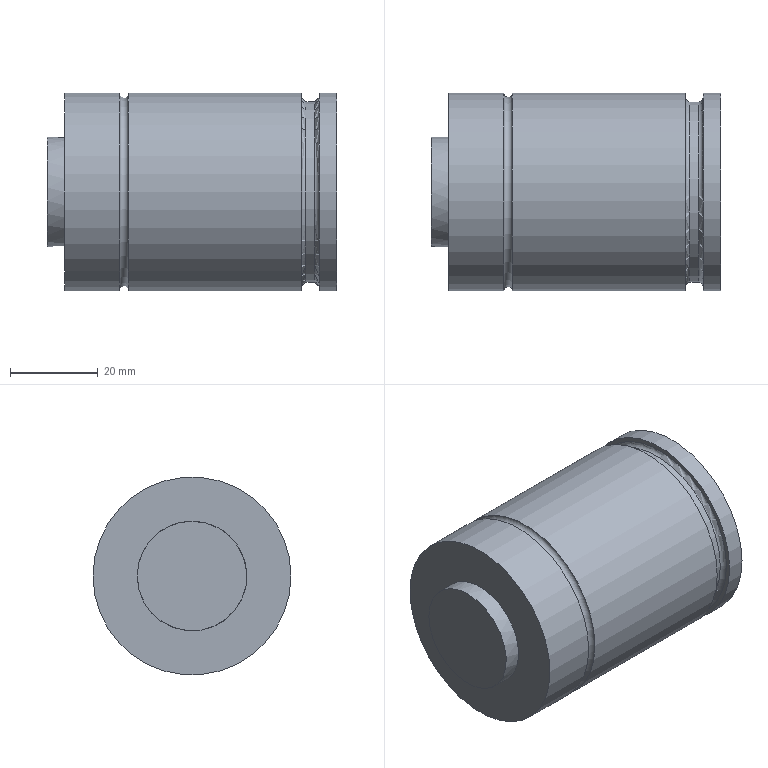Part | NX | features solid 2 | 1 solid | 17 faces | box 66 x 45.2 x 45.2 mm | volume 98109 mm3 | cylinder 7 | plane 5 | torus 3 | cone 2 | commonest cylinder face diameters 45.2 x3 8 x2 25 x1 41.2 x1
STEP:
#1=CARTESIAN_POINT('',(-246.5,-282.6,170.));
#2=VERTEX_POINT('',#1);
#3=CARTESIAN_POINT('',(-246.5,-260.,170.));
#4=DIRECTION('',(1.,0.,0.));
#5=DIRECTION('',(0.,-1.,0.));
#6=AXIS2_PLACEMENT_3D('',#3,#4,#5);
#7=CIRCLE('',#6,22.6);
#8=EDGE_CURVE('',#2,#2,#7,.T.);
#9=ORIENTED_EDGE('',*,*,#8,.T.);
#10=EDGE_LOOP('',(#9));
#11=FACE_BOUND('',#10,.T.);
#12=CARTESIAN_POINT('',(-207.,-237.4,170.));
#13=VERTEX_POINT('',#12);
#14=CARTESIAN_POINT('',(-207.,-260.,170.));
#15=DIRECTION('',(-1.,0.,0.));
#16=DIRECTION('',(0.,1.,0.));
#17=AXIS2_PLACEMENT_3D('',#14,#15,#16);
#18=CIRCLE('',#17,22.6);
#19=EDGE_CURVE('',#13,#13,#18,.T.);
#20=ORIENTED_EDGE('',*,*,#19,.T.);
#21=EDGE_LOOP('',(#20));
#22=FACE_BOUND('',#21,.T.);
#23=CARTESIAN_POINT('',(-261.,-260.,170.));
#24=DIRECTION('',(1.,0.,0.));
#25=DIRECTION('',(0.,-1.,0.));
#26=AXIS2_PLACEMENT_3D('',#23,#24,#25);
#27=CYLINDRICAL_SURFACE('',#26,22.6);
#28=ADVANCED_FACE('',(#11,#22),#27,.T.);
#29=CARTESIAN_POINT('',(-248.5,-282.6,170.));
#30=VERTEX_POINT('',#29);
#31=CARTESIAN_POINT('',(-248.5,-260.,170.));
#32=DIRECTION('',(1.,0.,0.));
#33=DIRECTION('',(0.,-1.,0.));
#34=AXIS2_PLACEMENT_3D('',#31,#32,#33);
#35=CIRCLE('',#34,22.6);
#36=EDGE_CURVE('',#30,#30,#35,.T.);
#37=ORIENTED_EDGE('',*,*,#36,.F.);
#38=EDGE_LOOP('',(#37));
#39=FACE_BOUND('',#38,.T.);
#40=CARTESIAN_POINT('',(-261.,-282.6,170.));
#41=VERTEX_POINT('',#40);
#42=CARTESIAN_POINT('',(-261.,-260.,170.));
#43=DIRECTION('',(1.,0.,0.));
#44=DIRECTION('',(0.,-1.,0.));
#45=AXIS2_PLACEMENT_3D('',#42,#43,#44);
#46=CIRCLE('',#45,22.6);
#47=EDGE_CURVE('',#41,#41,#46,.T.);
#48=ORIENTED_EDGE('',*,*,#47,.T.);
#49=EDGE_LOOP('',(#48));
#50=FACE_BOUND('',#49,.T.);
#51=CARTESIAN_POINT('',(-261.,-260.,170.));
#52=DIRECTION('',(1.,0.,0.));
#53=DIRECTION('',(0.,-1.,0.));
#54=AXIS2_PLACEMENT_3D('',#51,#52,#53);
#55=CYLINDRICAL_SURFACE('',#54,22.6);
#56=ADVANCED_FACE('',(#39,#50),#55,.T.);
#57=CARTESIAN_POINT('',(-261.,-247.5,170.));
#58=VERTEX_POINT('',#57);
#59=CARTESIAN_POINT('',(-261.,-260.,170.));
#60=DIRECTION('',(-1.,0.,0.));
#61=DIRECTION('',(0.,1.,0.));
#62=AXIS2_PLACEMENT_3D('',#59,#60,#61);
#63=CIRCLE('',#62,12.5);
#64=EDGE_CURVE('',#58,#58,#63,.T.);
#65=ORIENTED_EDGE('',*,*,#64,.F.);
#66=EDGE_LOOP('',(#65));
#67=FACE_BOUND('',#66,.T.);
#68=ORIENTED_EDGE('',*,*,#47,.F.);
#69=EDGE_LOOP('',(#68));
#70=FACE_BOUND('',#69,.T.);
#71=CARTESIAN_POINT('',(-261.,-260.,170.));
#72=DIRECTION('',(-1.,0.,0.));
#73=DIRECTION('',(0.,1.,0.));
#74=AXIS2_PLACEMENT_3D('',#71,#72,#73);
#75=PLANE('',#74);
#76=ADVANCED_FACE('',(#67,#70),#75,.T.);
#77=CARTESIAN_POINT('',(-265.,-260.,182.5));
#78=VERTEX_POINT('',#77);
#79=CARTESIAN_POINT('',(-265.,-260.,170.));
#80=DIRECTION('',(-1.,0.,0.));
#81=DIRECTION('',(0.,0.,1.));
#82=AXIS2_PLACEMENT_3D('',#79,#80,#81);
#83=CIRCLE('',#82,12.5);
#84=EDGE_CURVE('',#78,#78,#83,.F.);
#85=ORIENTED_EDGE('',*,*,#84,.F.);
#86=EDGE_LOOP('',(#85));
#87=FACE_BOUND('',#86,.T.);
#88=CARTESIAN_POINT('',(-265.,-260.,170.));
#89=DIRECTION('',(-1.,0.,0.));
#90=DIRECTION('',(0.,1.,0.));
#91=AXIS2_PLACEMENT_3D('',#88,#89,#90);
#92=PLANE('',#91);
#93=ADVANCED_FACE('',(#87),#92,.T.);
#94=ORIENTED_EDGE('',*,*,#84,.T.);
#95=EDGE_LOOP('',(#94));
#96=FACE_BOUND('',#95,.T.);
#97=ORIENTED_EDGE('',*,*,#64,.T.);
#98=EDGE_LOOP('',(#97));
#99=FACE_BOUND('',#98,.T.);
#100=CARTESIAN_POINT('',(-261.,-260.,170.));
#101=DIRECTION('',(-1.,0.,0.));
#102=DIRECTION('',(0.,1.,0.));
#103=AXIS2_PLACEMENT_3D('',#100,#101,#102);
#104=CYLINDRICAL_SURFACE('',#103,12.5);
#105=ADVANCED_FACE('',(#96,#99),#104,.T.);
#106=ORIENTED_EDGE('',*,*,#36,.T.);
#107=EDGE_LOOP('',(#106));
#108=FACE_BOUND('',#107,.T.);
#109=ORIENTED_EDGE('',*,*,#8,.F.);
#110=EDGE_LOOP('',(#109));
#111=FACE_BOUND('',#110,.T.);
#112=CARTESIAN_POINT('',(-247.5,-260.,170.));
#113=DIRECTION('',(-1.,0.,0.));
#114=DIRECTION('',(0.,1.,0.));
#115=AXIS2_PLACEMENT_3D('',#112,#113,#114);
#116=TOROIDAL_SURFACE('',#115,22.6,1.);
#117=ADVANCED_FACE('',(#108,#111),#116,.F.);
#118=CARTESIAN_POINT('',(-207.,-281.6,170.));
#119=VERTEX_POINT('',#118);
#120=CARTESIAN_POINT('',(-207.,-260.,170.));
#121=DIRECTION('',(1.,0.,0.));
#122=DIRECTION('',(0.,-1.,0.));
#123=AXIS2_PLACEMENT_3D('',#120,#121,#122);
#124=CIRCLE('',#123,21.6);
#125=EDGE_CURVE('',#119,#119,#124,.F.);
#126=ORIENTED_EDGE('',*,*,#125,.T.);
#127=EDGE_LOOP('',(#126));
#128=FACE_BOUND('',#127,.T.);
#129=ORIENTED_EDGE('',*,*,#19,.F.);
#130=EDGE_LOOP('',(#129));
#131=FACE_BOUND('',#130,.T.);
#132=CARTESIAN_POINT('',(-207.,-260.,170.));
#133=DIRECTION('',(1.,0.,0.));
#134=DIRECTION('',(0.,-1.,0.));
#135=AXIS2_PLACEMENT_3D('',#132,#133,#134);
#136=PLANE('',#135);
#137=ADVANCED_FACE('',(#128,#131),#136,.T.);
#138=CARTESIAN_POINT('',(-203.,-281.6,170.));
#139=VERTEX_POINT('',#138);
#140=CARTESIAN_POINT('',(-203.,-260.,170.));
#141=DIRECTION('',(1.,0.,0.));
#142=DIRECTION('',(0.,-1.,0.));
#143=AXIS2_PLACEMENT_3D('',#140,#141,#142);
#144=CIRCLE('',#143,21.6);
#145=EDGE_CURVE('',#139,#139,#144,.T.);
#146=ORIENTED_EDGE('',*,*,#145,.T.);
#147=EDGE_LOOP('',(#146));
#148=FACE_BOUND('',#147,.T.);
#149=CARTESIAN_POINT('',(-203.,-237.4,170.));
#150=VERTEX_POINT('',#149);
#151=CARTESIAN_POINT('',(-203.,-260.,170.));
#152=DIRECTION('',(-1.,0.,0.));
#153=DIRECTION('',(0.,1.,0.));
#154=AXIS2_PLACEMENT_3D('',#151,#152,#153);
#155=CIRCLE('',#154,22.6);
#156=EDGE_CURVE('',#150,#150,#155,.T.);
#157=ORIENTED_EDGE('',*,*,#156,.T.);
#158=EDGE_LOOP('',(#157));
#159=FACE_BOUND('',#158,.T.);
#160=CARTESIAN_POINT('',(-203.,-260.,170.));
#161=DIRECTION('',(1.,0.,0.));
#162=DIRECTION('',(0.,-1.,0.));
#163=AXIS2_PLACEMENT_3D('',#160,#161,#162);
#164=PLANE('',#163);
#165=ADVANCED_FACE('',(#148,#159),#164,.F.);
#166=CARTESIAN_POINT('',(-204.,-280.6,170.));
#167=VERTEX_POINT('',#166);
#168=CARTESIAN_POINT('',(-204.,-260.,170.));
#169=DIRECTION('',(1.,0.,0.));
#170=DIRECTION('',(0.,-1.,0.));
#171=AXIS2_PLACEMENT_3D('',#168,#169,#170);
#172=CIRCLE('',#171,20.6);
#173=EDGE_CURVE('',#167,#167,#172,.F.);
#174=ORIENTED_EDGE('',*,*,#173,.T.);
#175=EDGE_LOOP('',(#174));
#176=FACE_BOUND('',#175,.T.);
#177=CARTESIAN_POINT('',(-206.,-280.6,170.));
#178=VERTEX_POINT('',#177);
#179=CARTESIAN_POINT('',(-206.,-260.,170.));
#180=DIRECTION('',(1.,0.,0.));
#181=DIRECTION('',(0.,-1.,0.));
#182=AXIS2_PLACEMENT_3D('',#179,#180,#181);
#183=CIRCLE('',#182,20.6);
#184=EDGE_CURVE('',#178,#178,#183,.T.);
#185=ORIENTED_EDGE('',*,*,#184,.T.);
#186=EDGE_LOOP('',(#185));
#187=FACE_BOUND('',#186,.T.);
#188=CARTESIAN_POINT('',(-203.,-260.,170.));
#189=DIRECTION('',(-1.,0.,0.));
#190=DIRECTION('',(0.,1.,0.));
#191=AXIS2_PLACEMENT_3D('',#188,#189,#190);
#192=CYLINDRICAL_SURFACE('',#191,20.6);
#193=ADVANCED_FACE('',(#176,#187),#192,.T.);
#194=CARTESIAN_POINT('',(-199.,-250.,174.));
#195=VERTEX_POINT('',#194);
#196=CARTESIAN_POINT('',(-199.,-250.,170.));
#197=DIRECTION('',(-1.,0.,0.));
#198=DIRECTION('',(0.,0.,1.));
#199=AXIS2_PLACEMENT_3D('',#196,#197,#198);
#200=CIRCLE('',#199,4.);
#201=EDGE_CURVE('',#195,#195,#200,.T.);
#202=ORIENTED_EDGE('',*,*,#201,.T.);
#203=EDGE_LOOP('',(#202));
#204=FACE_BOUND('',#203,.T.);
#205=CARTESIAN_POINT('',(-199.,-270.,174.));
#206=VERTEX_POINT('',#205);
#207=CARTESIAN_POINT('',(-199.,-270.,170.));
#208=DIRECTION('',(-1.,0.,0.));
#209=DIRECTION('',(0.,0.,1.));
#210=AXIS2_PLACEMENT_3D('',#207,#208,#209);
#211=CIRCLE('',#210,4.);
#212=EDGE_CURVE('',#206,#206,#211,.T.);
#213=ORIENTED_EDGE('',*,*,#212,.T.);
#214=EDGE_LOOP('',(#213));
#215=FACE_BOUND('',#214,.T.);
#216=CARTESIAN_POINT('',(-199.,-237.4,170.));
#217=VERTEX_POINT('',#216);
#218=CARTESIAN_POINT('',(-199.,-260.,170.));
#219=DIRECTION('',(-1.,0.,0.));
#220=DIRECTION('',(0.,1.,0.));
#221=AXIS2_PLACEMENT_3D('',#218,#219,#220);
#222=CIRCLE('',#221,22.6);
#223=EDGE_CURVE('',#217,#217,#222,.T.);
#224=ORIENTED_EDGE('',*,*,#223,.F.);
#225=EDGE_LOOP('',(#224));
#226=FACE_BOUND('',#225,.T.);
#227=CARTESIAN_POINT('',(-199.,-260.,170.));
#228=DIRECTION('',(1.,0.,0.));
#229=DIRECTION('',(0.,-1.,0.));
#230=AXIS2_PLACEMENT_3D('',#227,#228,#229);
#231=PLANE('',#230);
#232=ADVANCED_FACE('',(#204,#215,#226),#231,.T.);
#233=ORIENTED_EDGE('',*,*,#223,.T.);
#234=EDGE_LOOP('',(#233));
#235=FACE_BOUND('',#234,.T.);
#236=ORIENTED_EDGE('',*,*,#156,.F.);
#237=EDGE_LOOP('',(#236));
#238=FACE_BOUND('',#237,.T.);
#239=CARTESIAN_POINT('',(-261.,-260.,170.));
#240=DIRECTION('',(1.,0.,0.));
#241=DIRECTION('',(0.,-1.,0.));
#242=AXIS2_PLACEMENT_3D('',#239,#240,#241);
#243=CYLINDRICAL_SURFACE('',#242,22.6);
#244=ADVANCED_FACE('',(#235,#238),#243,.T.);
#245=ORIENTED_EDGE('',*,*,#145,.F.);
#246=EDGE_LOOP('',(#245));
#247=FACE_BOUND('',#246,.T.);
#248=ORIENTED_EDGE('',*,*,#173,.F.);
#249=EDGE_LOOP('',(#248));
#250=FACE_BOUND('',#249,.T.);
#251=CARTESIAN_POINT('',(-204.,-260.,170.));
#252=DIRECTION('',(1.,0.,0.));
#253=DIRECTION('',(0.,-1.,0.));
#254=AXIS2_PLACEMENT_3D('',#251,#252,#253);
#255=TOROIDAL_SURFACE('',#254,21.6,1.);
#256=ADVANCED_FACE('',(#247,#250),#255,.F.);
#257=ORIENTED_EDGE('',*,*,#184,.F.);
#258=EDGE_LOOP('',(#257));
#259=FACE_BOUND('',#258,.T.);
#260=ORIENTED_EDGE('',*,*,#125,.F.);
#261=EDGE_LOOP('',(#260));
#262=FACE_BOUND('',#261,.T.);
#263=CARTESIAN_POINT('',(-206.,-260.,170.));
#264=DIRECTION('',(1.,0.,0.));
#265=DIRECTION('',(0.,-1.,0.));
#266=AXIS2_PLACEMENT_3D('',#263,#264,#265);
#267=TOROIDAL_SURFACE('',#266,21.6,1.);
#268=ADVANCED_FACE('',(#259,#262),#267,.F.);
#269=CARTESIAN_POINT('',(-219.,-270.,174.));
#270=VERTEX_POINT('',#269);
#271=CARTESIAN_POINT('',(-219.,-270.,170.));
#272=DIRECTION('',(-1.,0.,0.));
#273=DIRECTION('',(0.,0.,1.));
#274=AXIS2_PLACEMENT_3D('',#271,#272,#273);
#275=CIRCLE('',#274,4.);
#276=EDGE_CURVE('',#270,#270,#275,.T.);
#277=ORIENTED_EDGE('',*,*,#276,.F.);
#278=EDGE_LOOP('',(#277));
#279=FACE_BOUND('',#278,.T.);
#280=CARTESIAN_POINT('',(-221.403,-270.,170.));
#281=VERTEX_POINT('',#280);
#282=VERTEX_LOOP('',#281);
#283=FACE_BOUND('',#282,.T.);
#284=CARTESIAN_POINT('',(-219.,-270.,170.));
#285=DIRECTION('',(1.,0.,0.));
#286=DIRECTION('',(0.,0.,-1.));
#287=AXIS2_PLACEMENT_3D('',#284,#285,#286);
#288=CONICAL_SURFACE('',#287,4.,1.03);
#289=ADVANCED_FACE('',(#279,#283),#288,.F.);
#290=ORIENTED_EDGE('',*,*,#276,.T.);
#291=EDGE_LOOP('',(#290));
#292=FACE_BOUND('',#291,.T.);
#293=ORIENTED_EDGE('',*,*,#212,.F.);
#294=EDGE_LOOP('',(#293));
#295=FACE_BOUND('',#294,.T.);
#296=CARTESIAN_POINT('',(-199.,-270.,170.));
#297=DIRECTION('',(-1.,0.,0.));
#298=DIRECTION('',(0.,0.,1.));
#299=AXIS2_PLACEMENT_3D('',#296,#297,#298);
#300=CYLINDRICAL_SURFACE('',#299,4.);
#301=ADVANCED_FACE('',(#292,#295),#300,.F.);
#302=CARTESIAN_POINT('',(-219.,-250.,174.));
#303=VERTEX_POINT('',#302);
#304=CARTESIAN_POINT('',(-219.,-250.,170.));
#305=DIRECTION('',(-1.,0.,0.));
#306=DIRECTION('',(0.,0.,1.));
#307=AXIS2_PLACEMENT_3D('',#304,#305,#306);
#308=CIRCLE('',#307,4.);
#309=EDGE_CURVE('',#303,#303,#308,.T.);
#310=ORIENTED_EDGE('',*,*,#309,.F.);
#311=EDGE_LOOP('',(#310));
#312=FACE_BOUND('',#311,.T.);
#313=CARTESIAN_POINT('',(-221.403,-250.,170.));
#314=VERTEX_POINT('',#313);
#315=VERTEX_LOOP('',#314);
#316=FACE_BOUND('',#315,.T.);
#317=CARTESIAN_POINT('',(-219.,-250.,170.));
#318=DIRECTION('',(1.,0.,0.));
#319=DIRECTION('',(0.,0.,-1.));
#320=AXIS2_PLACEMENT_3D('',#317,#318,#319);
#321=CONICAL_SURFACE('',#320,4.,1.03);
#322=ADVANCED_FACE('',(#312,#316),#321,.F.);
#323=ORIENTED_EDGE('',*,*,#309,.T.);
#324=EDGE_LOOP('',(#323));
#325=FACE_BOUND('',#324,.T.);
#326=ORIENTED_EDGE('',*,*,#201,.F.);
#327=EDGE_LOOP('',(#326));
#328=FACE_BOUND('',#327,.T.);
#329=CARTESIAN_POINT('',(-199.,-250.,170.));
#330=DIRECTION('',(-1.,0.,0.));
#331=DIRECTION('',(0.,0.,1.));
#332=AXIS2_PLACEMENT_3D('',#329,#330,#331);
#333=CYLINDRICAL_SURFACE('',#332,4.);
#334=ADVANCED_FACE('',(#325,#328),#333,.F.);
#335=CLOSED_SHELL('',(#28,#56,#76,#93,#105,#117,#137,#165,#193,#232,#244,#256,#268,#289,#301,#322,#334));
#336=MANIFOLD_SOLID_BREP('',#335);
#337=(LENGTH_UNIT()NAMED_UNIT(*)SI_UNIT(.MILLI.,.METRE.));
#338=UNCERTAINTY_MEASURE_WITH_UNIT(LENGTH_MEASURE(0.00001),#337,'','');
#339=(NAMED_UNIT(*)PLANE_ANGLE_UNIT()SI_UNIT($,.RADIAN.));
#340=(NAMED_UNIT(*)SI_UNIT($,.STERADIAN.)SOLID_ANGLE_UNIT());
#341=(GEOMETRIC_REPRESENTATION_CONTEXT(3)GLOBAL_UNCERTAINTY_ASSIGNED_CONTEXT((#338))GLOBAL_UNIT_ASSIGNED_CONTEXT((#337,#339,#340))REPRESENTATION_CONTEXT('',''));
#342=ADVANCED_BREP_SHAPE_REPRESENTATION('',(#336),#341);